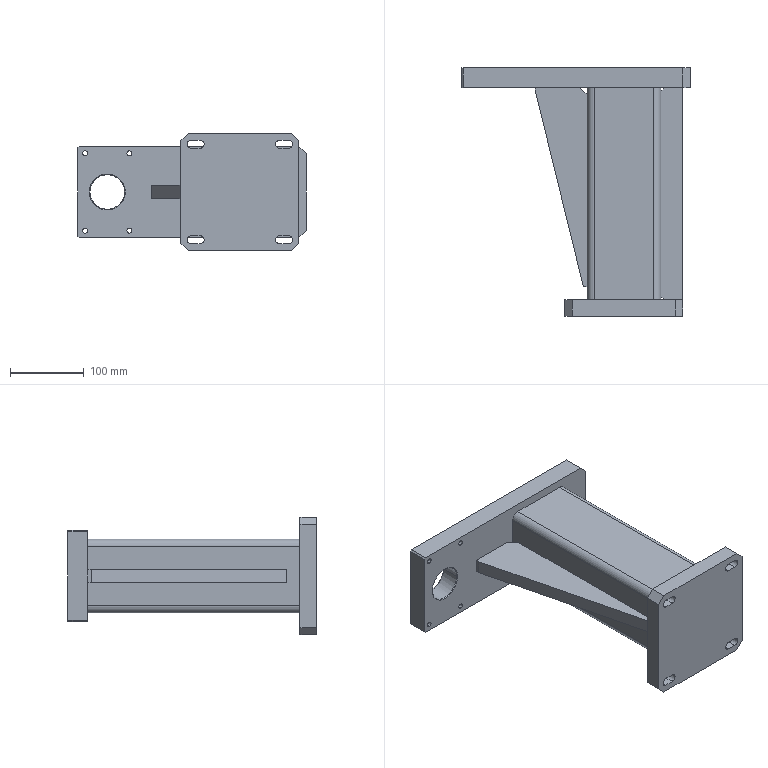Part | STEP file | PN_0003 Load-bearing support rod_default_machined_ | 5 solids | 84 faces | box 310 x 337 x 160 mm | volume 2390981 mm3 | plane 54 | cylinder 26 | cone 4 | commonest cylinder face diameters 6.8 x8 11 x8 10 x4 20 x4 47 x2